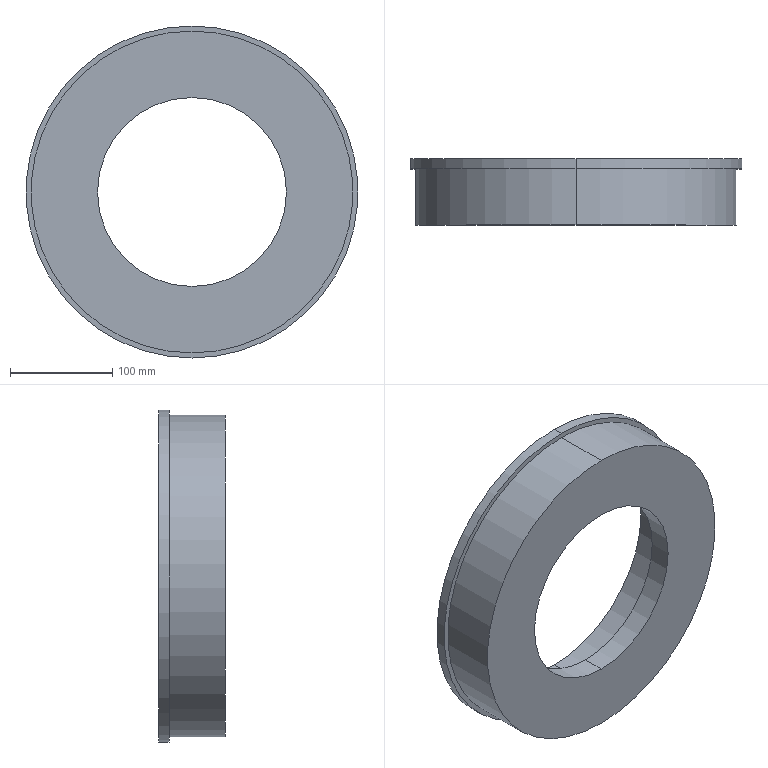Part | SolidWorks | features BaseBody 1 | 1 solid | 12 faces | box 325 x 65 x 325 mm | volume 2579149 mm3 | cylinder 8 | plane 4 | commonest cylinder face diameters 185 x2 240 x2 315 x2 325 x2
STEP:
#1=CARTESIAN_POINT('',(0.,55.,-157.5));
#2=VERTEX_POINT('',#1);
#3=CARTESIAN_POINT('',(0.,55.,157.5));
#4=VERTEX_POINT('',#3);
#5=CARTESIAN_POINT('',(0.,55.,0.));
#6=DIRECTION('',(0.,-1.,0.));
#7=DIRECTION('',(0.,0.,-1.));
#8=AXIS2_PLACEMENT_3D('',#5,#6,#7);
#9=CIRCLE('',#8,157.5);
#10=EDGE_CURVE('',#2,#4,#9,.T.);
#11=ORIENTED_EDGE('',*,*,#10,.T.);
#12=CARTESIAN_POINT('',(0.,0.,157.5));
#13=VERTEX_POINT('',#12);
#14=CARTESIAN_POINT('',(0.,55.,157.5));
#15=DIRECTION('',(0.,-1.,0.));
#16=VECTOR('',#15,1000.);
#17=LINE('',#14,#16);
#18=EDGE_CURVE('',#4,#13,#17,.T.);
#19=ORIENTED_EDGE('',*,*,#18,.T.);
#20=CARTESIAN_POINT('',(0.,0.,-157.5));
#21=VERTEX_POINT('',#20);
#22=CARTESIAN_POINT('',(0.,0.,0.));
#23=DIRECTION('',(0.,-1.,0.));
#24=DIRECTION('',(0.,0.,-1.));
#25=AXIS2_PLACEMENT_3D('',#22,#23,#24);
#26=CIRCLE('',#25,157.5);
#27=EDGE_CURVE('',#21,#13,#26,.T.);
#28=ORIENTED_EDGE('',*,*,#27,.F.);
#29=CARTESIAN_POINT('',(0.,55.,-157.5));
#30=DIRECTION('',(0.,-1.,0.));
#31=VECTOR('',#30,1000.);
#32=LINE('',#29,#31);
#33=EDGE_CURVE('',#2,#21,#32,.T.);
#34=ORIENTED_EDGE('',*,*,#33,.F.);
#35=EDGE_LOOP('',(#11,#19,#28,#34));
#36=FACE_OUTER_BOUND('',#35,.T.);
#37=CARTESIAN_POINT('',(0.,55.,0.));
#38=DIRECTION('',(0.,-1.,0.));
#39=DIRECTION('',(0.,0.,-1.));
#40=AXIS2_PLACEMENT_3D('',#37,#38,#39);
#41=CYLINDRICAL_SURFACE('',#40,157.5);
#42=ADVANCED_FACE('',(#36),#41,.T.);
#43=CARTESIAN_POINT('',(0.,0.,-92.5));
#44=VERTEX_POINT('',#43);
#45=CARTESIAN_POINT('',(0.,0.,92.5));
#46=VERTEX_POINT('',#45);
#47=CARTESIAN_POINT('',(0.,0.,0.));
#48=DIRECTION('',(0.,1.,0.));
#49=DIRECTION('',(0.,0.,1.));
#50=AXIS2_PLACEMENT_3D('',#47,#48,#49);
#51=CIRCLE('',#50,92.5);
#52=EDGE_CURVE('',#44,#46,#51,.T.);
#53=ORIENTED_EDGE('',*,*,#52,.F.);
#54=CARTESIAN_POINT('',(0.,22.,-92.5));
#55=VERTEX_POINT('',#54);
#56=CARTESIAN_POINT('',(0.,0.,-92.5));
#57=DIRECTION('',(0.,1.,0.));
#58=VECTOR('',#57,1000.);
#59=LINE('',#56,#58);
#60=EDGE_CURVE('',#44,#55,#59,.T.);
#61=ORIENTED_EDGE('',*,*,#60,.T.);
#62=CARTESIAN_POINT('',(0.,22.,92.5));
#63=VERTEX_POINT('',#62);
#64=CARTESIAN_POINT('',(0.,22.,0.));
#65=DIRECTION('',(0.,1.,0.));
#66=DIRECTION('',(0.,0.,1.));
#67=AXIS2_PLACEMENT_3D('',#64,#65,#66);
#68=CIRCLE('',#67,92.5);
#69=EDGE_CURVE('',#55,#63,#68,.T.);
#70=ORIENTED_EDGE('',*,*,#69,.T.);
#71=CARTESIAN_POINT('',(0.,0.,92.5));
#72=DIRECTION('',(0.,1.,0.));
#73=VECTOR('',#72,1000.);
#74=LINE('',#71,#73);
#75=EDGE_CURVE('',#46,#63,#74,.T.);
#76=ORIENTED_EDGE('',*,*,#75,.F.);
#77=EDGE_LOOP('',(#53,#61,#70,#76));
#78=FACE_OUTER_BOUND('',#77,.T.);
#79=CARTESIAN_POINT('',(0.,0.,0.));
#80=DIRECTION('',(0.,1.,0.));
#81=DIRECTION('',(0.,0.,1.));
#82=AXIS2_PLACEMENT_3D('',#79,#80,#81);
#83=CYLINDRICAL_SURFACE('',#82,92.5);
#84=ADVANCED_FACE('',(#78),#83,.F.);
#85=CARTESIAN_POINT('',(0.,22.,-120.));
#86=VERTEX_POINT('',#85);
#87=CARTESIAN_POINT('',(0.,22.,120.));
#88=VERTEX_POINT('',#87);
#89=CARTESIAN_POINT('',(0.,22.,0.));
#90=DIRECTION('',(0.,1.,0.));
#91=DIRECTION('',(0.,0.,1.));
#92=AXIS2_PLACEMENT_3D('',#89,#90,#91);
#93=CIRCLE('',#92,120.);
#94=EDGE_CURVE('',#86,#88,#93,.T.);
#95=ORIENTED_EDGE('',*,*,#94,.F.);
#96=CARTESIAN_POINT('',(0.,65.,-120.));
#97=VERTEX_POINT('',#96);
#98=CARTESIAN_POINT('',(0.,22.,-120.));
#99=DIRECTION('',(0.,1.,0.));
#100=VECTOR('',#99,1000.);
#101=LINE('',#98,#100);
#102=EDGE_CURVE('',#86,#97,#101,.T.);
#103=ORIENTED_EDGE('',*,*,#102,.T.);
#104=CARTESIAN_POINT('',(0.,65.,120.));
#105=VERTEX_POINT('',#104);
#106=CARTESIAN_POINT('',(0.,65.,0.));
#107=DIRECTION('',(0.,1.,0.));
#108=DIRECTION('',(0.,0.,1.));
#109=AXIS2_PLACEMENT_3D('',#106,#107,#108);
#110=CIRCLE('',#109,120.);
#111=EDGE_CURVE('',#97,#105,#110,.T.);
#112=ORIENTED_EDGE('',*,*,#111,.T.);
#113=CARTESIAN_POINT('',(0.,22.,120.));
#114=DIRECTION('',(0.,1.,0.));
#115=VECTOR('',#114,1000.);
#116=LINE('',#113,#115);
#117=EDGE_CURVE('',#88,#105,#116,.T.);
#118=ORIENTED_EDGE('',*,*,#117,.F.);
#119=EDGE_LOOP('',(#95,#103,#112,#118));
#120=FACE_OUTER_BOUND('',#119,.T.);
#121=CARTESIAN_POINT('',(0.,22.,0.));
#122=DIRECTION('',(0.,1.,0.));
#123=DIRECTION('',(0.,0.,1.));
#124=AXIS2_PLACEMENT_3D('',#121,#122,#123);
#125=CYLINDRICAL_SURFACE('',#124,120.);
#126=ADVANCED_FACE('',(#120),#125,.F.);
#127=CARTESIAN_POINT('',(0.,65.,162.5));
#128=VERTEX_POINT('',#127);
#129=CARTESIAN_POINT('',(0.,65.,-162.5));
#130=VERTEX_POINT('',#129);
#131=CARTESIAN_POINT('',(0.,65.,0.));
#132=DIRECTION('',(0.,1.,0.));
#133=DIRECTION('',(0.,0.,1.));
#134=AXIS2_PLACEMENT_3D('',#131,#132,#133);
#135=CIRCLE('',#134,162.5);
#136=EDGE_CURVE('',#128,#130,#135,.T.);
#137=ORIENTED_EDGE('',*,*,#136,.F.);
#138=CARTESIAN_POINT('',(0.,55.,162.5));
#139=VERTEX_POINT('',#138);
#140=CARTESIAN_POINT('',(0.,65.,162.5));
#141=DIRECTION('',(0.,-1.,0.));
#142=VECTOR('',#141,1000.);
#143=LINE('',#140,#142);
#144=EDGE_CURVE('',#128,#139,#143,.T.);
#145=ORIENTED_EDGE('',*,*,#144,.T.);
#146=CARTESIAN_POINT('',(0.,55.,-162.5));
#147=VERTEX_POINT('',#146);
#148=CARTESIAN_POINT('',(0.,55.,0.));
#149=DIRECTION('',(0.,-1.,0.));
#150=DIRECTION('',(0.,0.,-1.));
#151=AXIS2_PLACEMENT_3D('',#148,#149,#150);
#152=CIRCLE('',#151,162.5);
#153=EDGE_CURVE('',#147,#139,#152,.T.);
#154=ORIENTED_EDGE('',*,*,#153,.F.);
#155=CARTESIAN_POINT('',(0.,65.,-162.5));
#156=DIRECTION('',(0.,-1.,0.));
#157=VECTOR('',#156,1000.);
#158=LINE('',#155,#157);
#159=EDGE_CURVE('',#130,#147,#158,.T.);
#160=ORIENTED_EDGE('',*,*,#159,.F.);
#161=EDGE_LOOP('',(#137,#145,#154,#160));
#162=FACE_OUTER_BOUND('',#161,.T.);
#163=CARTESIAN_POINT('',(0.,65.,0.));
#164=DIRECTION('',(0.,-1.,0.));
#165=DIRECTION('',(0.,0.,-1.));
#166=AXIS2_PLACEMENT_3D('',#163,#164,#165);
#167=CYLINDRICAL_SURFACE('',#166,162.5);
#168=ADVANCED_FACE('',(#162),#167,.T.);
#169=ORIENTED_EDGE('',*,*,#144,.F.);
#170=CARTESIAN_POINT('',(0.,65.,0.));
#171=DIRECTION('',(0.,1.,0.));
#172=DIRECTION('',(0.,0.,1.));
#173=AXIS2_PLACEMENT_3D('',#170,#171,#172);
#174=CIRCLE('',#173,162.5);
#175=EDGE_CURVE('',#130,#128,#174,.T.);
#176=ORIENTED_EDGE('',*,*,#175,.F.);
#177=ORIENTED_EDGE('',*,*,#159,.T.);
#178=CARTESIAN_POINT('',(0.,55.,0.));
#179=DIRECTION('',(0.,-1.,0.));
#180=DIRECTION('',(0.,0.,-1.));
#181=AXIS2_PLACEMENT_3D('',#178,#179,#180);
#182=CIRCLE('',#181,162.5);
#183=EDGE_CURVE('',#139,#147,#182,.T.);
#184=ORIENTED_EDGE('',*,*,#183,.F.);
#185=EDGE_LOOP('',(#169,#176,#177,#184));
#186=FACE_OUTER_BOUND('',#185,.T.);
#187=CARTESIAN_POINT('',(0.,65.,0.));
#188=DIRECTION('',(0.,-1.,0.));
#189=DIRECTION('',(0.,0.,-1.));
#190=AXIS2_PLACEMENT_3D('',#187,#188,#189);
#191=CYLINDRICAL_SURFACE('',#190,162.5);
#192=ADVANCED_FACE('',(#186),#191,.T.);
#193=CARTESIAN_POINT('',(0.,0.,0.));
#194=DIRECTION('',(0.,1.,0.));
#195=DIRECTION('',(0.,0.,1.));
#196=AXIS2_PLACEMENT_3D('',#193,#194,#195);
#197=CIRCLE('',#196,92.5);
#198=EDGE_CURVE('',#46,#44,#197,.T.);
#199=ORIENTED_EDGE('',*,*,#198,.T.);
#200=ORIENTED_EDGE('',*,*,#52,.T.);
#201=EDGE_LOOP('',(#199,#200));
#202=FACE_BOUND('',#201,.T.);
#203=ORIENTED_EDGE('',*,*,#27,.T.);
#204=CARTESIAN_POINT('',(0.,0.,0.));
#205=DIRECTION('',(0.,-1.,0.));
#206=DIRECTION('',(0.,0.,-1.));
#207=AXIS2_PLACEMENT_3D('',#204,#205,#206);
#208=CIRCLE('',#207,157.5);
#209=EDGE_CURVE('',#13,#21,#208,.T.);
#210=ORIENTED_EDGE('',*,*,#209,.T.);
#211=EDGE_LOOP('',(#203,#210));
#212=FACE_OUTER_BOUND('',#211,.T.);
#213=CARTESIAN_POINT('',(0.,0.,0.));
#214=DIRECTION('',(0.,1.,0.));
#215=DIRECTION('',(0.,0.,1.));
#216=AXIS2_PLACEMENT_3D('',#213,#214,#215);
#217=PLANE('',#216);
#218=ADVANCED_FACE('',(#202,#212),#217,.F.);
#219=CARTESIAN_POINT('',(0.,65.,0.));
#220=DIRECTION('',(0.,1.,0.));
#221=DIRECTION('',(0.,0.,1.));
#222=AXIS2_PLACEMENT_3D('',#219,#220,#221);
#223=CIRCLE('',#222,120.);
#224=EDGE_CURVE('',#105,#97,#223,.T.);
#225=ORIENTED_EDGE('',*,*,#224,.F.);
#226=ORIENTED_EDGE('',*,*,#111,.F.);
#227=EDGE_LOOP('',(#225,#226));
#228=FACE_BOUND('',#227,.T.);
#229=ORIENTED_EDGE('',*,*,#175,.T.);
#230=ORIENTED_EDGE('',*,*,#136,.T.);
#231=EDGE_LOOP('',(#229,#230));
#232=FACE_OUTER_BOUND('',#231,.T.);
#233=CARTESIAN_POINT('',(0.,65.,0.));
#234=DIRECTION('',(0.,1.,0.));
#235=DIRECTION('',(0.,0.,1.));
#236=AXIS2_PLACEMENT_3D('',#233,#234,#235);
#237=PLANE('',#236);
#238=ADVANCED_FACE('',(#228,#232),#237,.T.);
#239=ORIENTED_EDGE('',*,*,#102,.F.);
#240=CARTESIAN_POINT('',(0.,22.,0.));
#241=DIRECTION('',(0.,1.,0.));
#242=DIRECTION('',(0.,0.,1.));
#243=AXIS2_PLACEMENT_3D('',#240,#241,#242);
#244=CIRCLE('',#243,120.);
#245=EDGE_CURVE('',#88,#86,#244,.T.);
#246=ORIENTED_EDGE('',*,*,#245,.F.);
#247=ORIENTED_EDGE('',*,*,#117,.T.);
#248=ORIENTED_EDGE('',*,*,#224,.T.);
#249=EDGE_LOOP('',(#239,#246,#247,#248));
#250=FACE_OUTER_BOUND('',#249,.T.);
#251=CARTESIAN_POINT('',(0.,22.,0.));
#252=DIRECTION('',(0.,1.,0.));
#253=DIRECTION('',(0.,0.,1.));
#254=AXIS2_PLACEMENT_3D('',#251,#252,#253);
#255=CYLINDRICAL_SURFACE('',#254,120.);
#256=ADVANCED_FACE('',(#250),#255,.F.);
#257=CARTESIAN_POINT('',(0.,22.,0.));
#258=DIRECTION('',(0.,1.,0.));
#259=DIRECTION('',(0.,0.,1.));
#260=AXIS2_PLACEMENT_3D('',#257,#258,#259);
#261=CIRCLE('',#260,92.5);
#262=EDGE_CURVE('',#63,#55,#261,.T.);
#263=ORIENTED_EDGE('',*,*,#262,.F.);
#264=ORIENTED_EDGE('',*,*,#69,.F.);
#265=EDGE_LOOP('',(#263,#264));
#266=FACE_BOUND('',#265,.T.);
#267=ORIENTED_EDGE('',*,*,#245,.T.);
#268=ORIENTED_EDGE('',*,*,#94,.T.);
#269=EDGE_LOOP('',(#267,#268));
#270=FACE_OUTER_BOUND('',#269,.T.);
#271=CARTESIAN_POINT('',(0.,22.,0.));
#272=DIRECTION('',(0.,1.,0.));
#273=DIRECTION('',(0.,0.,1.));
#274=AXIS2_PLACEMENT_3D('',#271,#272,#273);
#275=PLANE('',#274);
#276=ADVANCED_FACE('',(#266,#270),#275,.T.);
#277=ORIENTED_EDGE('',*,*,#60,.F.);
#278=ORIENTED_EDGE('',*,*,#198,.F.);
#279=ORIENTED_EDGE('',*,*,#75,.T.);
#280=ORIENTED_EDGE('',*,*,#262,.T.);
#281=EDGE_LOOP('',(#277,#278,#279,#280));
#282=FACE_OUTER_BOUND('',#281,.T.);
#283=CARTESIAN_POINT('',(0.,0.,0.));
#284=DIRECTION('',(0.,1.,0.));
#285=DIRECTION('',(0.,0.,1.));
#286=AXIS2_PLACEMENT_3D('',#283,#284,#285);
#287=CYLINDRICAL_SURFACE('',#286,92.5);
#288=ADVANCED_FACE('',(#282),#287,.F.);
#289=ORIENTED_EDGE('',*,*,#10,.F.);
#290=CARTESIAN_POINT('',(0.,55.,0.));
#291=DIRECTION('',(0.,-1.,0.));
#292=DIRECTION('',(0.,0.,-1.));
#293=AXIS2_PLACEMENT_3D('',#290,#291,#292);
#294=CIRCLE('',#293,157.5);
#295=EDGE_CURVE('',#4,#2,#294,.T.);
#296=ORIENTED_EDGE('',*,*,#295,.F.);
#297=EDGE_LOOP('',(#289,#296));
#298=FACE_BOUND('',#297,.T.);
#299=ORIENTED_EDGE('',*,*,#153,.T.);
#300=ORIENTED_EDGE('',*,*,#183,.T.);
#301=EDGE_LOOP('',(#299,#300));
#302=FACE_OUTER_BOUND('',#301,.T.);
#303=CARTESIAN_POINT('',(0.,55.,0.));
#304=DIRECTION('',(0.,-1.,0.));
#305=DIRECTION('',(0.,0.,-1.));
#306=AXIS2_PLACEMENT_3D('',#303,#304,#305);
#307=PLANE('',#306);
#308=ADVANCED_FACE('',(#298,#302),#307,.T.);
#309=ORIENTED_EDGE('',*,*,#18,.F.);
#310=ORIENTED_EDGE('',*,*,#295,.T.);
#311=ORIENTED_EDGE('',*,*,#33,.T.);
#312=ORIENTED_EDGE('',*,*,#209,.F.);
#313=EDGE_LOOP('',(#309,#310,#311,#312));
#314=FACE_OUTER_BOUND('',#313,.T.);
#315=CARTESIAN_POINT('',(0.,55.,0.));
#316=DIRECTION('',(0.,-1.,0.));
#317=DIRECTION('',(0.,0.,-1.));
#318=AXIS2_PLACEMENT_3D('',#315,#316,#317);
#319=CYLINDRICAL_SURFACE('',#318,157.5);
#320=ADVANCED_FACE('',(#314),#319,.T.);
#321=CLOSED_SHELL('',(#42,#84,#126,#168,#192,#218,#238,#256,#276,#288,#308,#320));
#322=MANIFOLD_SOLID_BREP('',#321);
#323=CARTESIAN_POINT('',(0.,0.,0.));
#324=DIRECTION('',(0.,0.,1.));
#325=DIRECTION('',(1.,0.,0.));
#326=AXIS2_PLACEMENT_3D('',#323,#324,#325);
#327=(LENGTH_UNIT()NAMED_UNIT(*)SI_UNIT(.MILLI.,.METRE.));
#328=UNCERTAINTY_MEASURE_WITH_UNIT(LENGTH_MEASURE(0.00001),#327,'','');
#329=(NAMED_UNIT(*)PLANE_ANGLE_UNIT()SI_UNIT($,.RADIAN.));
#330=(NAMED_UNIT(*)SI_UNIT($,.STERADIAN.)SOLID_ANGLE_UNIT());
#331=(GEOMETRIC_REPRESENTATION_CONTEXT(3)GLOBAL_UNCERTAINTY_ASSIGNED_CONTEXT((#328))GLOBAL_UNIT_ASSIGNED_CONTEXT((#327,#329,#330))REPRESENTATION_CONTEXT('',''));
#332=ADVANCED_BREP_SHAPE_REPRESENTATION('',(#322,#326),#331);